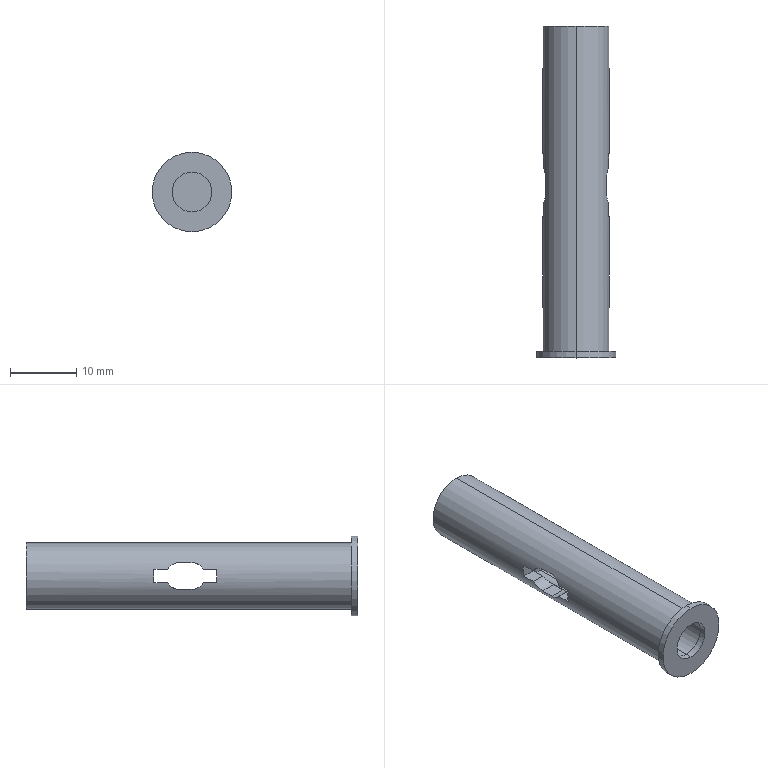Part | SolidWorks | features ICE 3, Revolution 1 | 1 solid | 37 faces | box 12 x 50 x 12 mm | volume 2925 mm3 | plane 21 | cylinder 16 | commonest cylinder face diameters 4 x8 6 x2 6.05 x2 10 x2 12 x2
STEP:
#1=CARTESIAN_POINT('',(0.,1.,-3.));
#2=VERTEX_POINT('',#1);
#3=CARTESIAN_POINT('',(0.,1.,3.));
#4=VERTEX_POINT('',#3);
#5=CARTESIAN_POINT('',(0.,1.,0.));
#6=DIRECTION('',(0.,1.,0.));
#7=DIRECTION('',(0.,0.,1.));
#8=AXIS2_PLACEMENT_3D('',#5,#6,#7);
#9=CIRCLE('',#8,3.);
#10=EDGE_CURVE('',#2,#4,#9,.T.);
#11=ORIENTED_EDGE('',*,*,#10,.T.);
#12=CARTESIAN_POINT('',(0.,0.,3.));
#13=VERTEX_POINT('',#12);
#14=CARTESIAN_POINT('',(0.,1.,3.));
#15=DIRECTION('',(0.,-1.,0.));
#16=VECTOR('',#15,1000.);
#17=LINE('',#14,#16);
#18=EDGE_CURVE('',#4,#13,#17,.T.);
#19=ORIENTED_EDGE('',*,*,#18,.T.);
#20=CARTESIAN_POINT('',(0.,0.,-3.));
#21=VERTEX_POINT('',#20);
#22=CARTESIAN_POINT('',(0.,0.,0.));
#23=DIRECTION('',(0.,1.,0.));
#24=DIRECTION('',(0.,0.,1.));
#25=AXIS2_PLACEMENT_3D('',#22,#23,#24);
#26=CIRCLE('',#25,3.);
#27=EDGE_CURVE('',#21,#13,#26,.T.);
#28=ORIENTED_EDGE('',*,*,#27,.F.);
#29=CARTESIAN_POINT('',(0.,1.,-3.));
#30=DIRECTION('',(0.,-1.,0.));
#31=VECTOR('',#30,1000.);
#32=LINE('',#29,#31);
#33=EDGE_CURVE('',#2,#21,#32,.T.);
#34=ORIENTED_EDGE('',*,*,#33,.F.);
#35=EDGE_LOOP('',(#11,#19,#28,#34));
#36=FACE_OUTER_BOUND('',#35,.T.);
#37=CARTESIAN_POINT('',(0.,1.,0.));
#38=DIRECTION('',(0.,-1.,0.));
#39=DIRECTION('',(0.,0.,-1.));
#40=AXIS2_PLACEMENT_3D('',#37,#38,#39);
#41=CYLINDRICAL_SURFACE('',#40,3.);
#42=ADVANCED_FACE('',(#36),#41,.F.);
#43=CARTESIAN_POINT('',(0.,1.,6.));
#44=VERTEX_POINT('',#43);
#45=CARTESIAN_POINT('',(0.,1.,-6.));
#46=VERTEX_POINT('',#45);
#47=CARTESIAN_POINT('',(0.,1.,0.));
#48=DIRECTION('',(0.,1.,0.));
#49=DIRECTION('',(0.,0.,1.));
#50=AXIS2_PLACEMENT_3D('',#47,#48,#49);
#51=CIRCLE('',#50,6.);
#52=EDGE_CURVE('',#44,#46,#51,.T.);
#53=ORIENTED_EDGE('',*,*,#52,.F.);
#54=CARTESIAN_POINT('',(0.,0.,6.));
#55=VERTEX_POINT('',#54);
#56=CARTESIAN_POINT('',(0.,1.,6.));
#57=DIRECTION('',(0.,-1.,0.));
#58=VECTOR('',#57,1000.);
#59=LINE('',#56,#58);
#60=EDGE_CURVE('',#44,#55,#59,.T.);
#61=ORIENTED_EDGE('',*,*,#60,.T.);
#62=CARTESIAN_POINT('',(0.,0.,-6.));
#63=VERTEX_POINT('',#62);
#64=CARTESIAN_POINT('',(0.,0.,0.));
#65=DIRECTION('',(0.,1.,0.));
#66=DIRECTION('',(0.,0.,1.));
#67=AXIS2_PLACEMENT_3D('',#64,#65,#66);
#68=CIRCLE('',#67,6.);
#69=EDGE_CURVE('',#55,#63,#68,.T.);
#70=ORIENTED_EDGE('',*,*,#69,.T.);
#71=CARTESIAN_POINT('',(0.,1.,-6.));
#72=DIRECTION('',(0.,-1.,0.));
#73=VECTOR('',#72,1000.);
#74=LINE('',#71,#73);
#75=EDGE_CURVE('',#46,#63,#74,.T.);
#76=ORIENTED_EDGE('',*,*,#75,.F.);
#77=EDGE_LOOP('',(#53,#61,#70,#76));
#78=FACE_OUTER_BOUND('',#77,.T.);
#79=CARTESIAN_POINT('',(0.,1.,0.));
#80=DIRECTION('',(0.,-1.,0.));
#81=DIRECTION('',(0.,0.,-1.));
#82=AXIS2_PLACEMENT_3D('',#79,#80,#81);
#83=CYLINDRICAL_SURFACE('',#82,6.);
#84=ADVANCED_FACE('',(#78),#83,.T.);
#85=CARTESIAN_POINT('',(4.899,30.732,-1.));
#86=VERTEX_POINT('',#85);
#87=CARTESIAN_POINT('',(4.899,30.732,1.));
#88=VERTEX_POINT('',#87);
#89=CARTESIAN_POINT('',(0.,30.732,0.));
#90=DIRECTION('',(0.,-1.,0.));
#91=DIRECTION('',(0.,0.,1.));
#92=AXIS2_PLACEMENT_3D('',#89,#90,#91);
#93=CIRCLE('',#92,5.);
#94=EDGE_CURVE('',#86,#88,#93,.T.);
#95=ORIENTED_EDGE('',*,*,#94,.F.);
#96=CARTESIAN_POINT('',(4.899,28.732,-1.));
#97=VERTEX_POINT('',#96);
#98=CARTESIAN_POINT('',(4.899,-0.7297,-1.));
#99=DIRECTION('',(0.,1.,0.));
#100=VECTOR('',#99,1000.);
#101=LINE('',#98,#100);
#102=EDGE_CURVE('',#97,#86,#101,.T.);
#103=ORIENTED_EDGE('',*,*,#102,.F.);
#104=CARTESIAN_POINT('',(4.583,27.,-2.));
#105=VERTEX_POINT('',#104);
#106=CARTESIAN_POINT('',(4.583,27.,-2.));
#107=CARTESIAN_POINT('',(4.583,27.179,-2.));
#108=CARTESIAN_POINT('',(4.593,27.353,-1.977));
#109=CARTESIAN_POINT('',(4.631,27.692,-1.885));
#110=CARTESIAN_POINT('',(4.659,27.855,-1.816));
#111=CARTESIAN_POINT('',(4.724,28.155,-1.642));
#112=CARTESIAN_POINT('',(4.761,28.295,-1.534));
#113=CARTESIAN_POINT('',(4.832,28.538,-1.29));
#114=CARTESIAN_POINT('',(4.868,28.645,-1.15));
#115=CARTESIAN_POINT('',(4.899,28.732,-1.));
#116=B_SPLINE_CURVE_WITH_KNOTS('',3,(#106,#107,#108,#109,#110,#111,#112,#113,#114,#115),.UNSPECIFIED.,.F.,.F.,(4,2,2,2,4),(0.,0.0005276,0.001055,0.001583,0.00211),.UNSPECIFIED.);
#117=EDGE_CURVE('',#105,#97,#116,.T.);
#118=ORIENTED_EDGE('',*,*,#117,.F.);
#119=CARTESIAN_POINT('',(4.583,25.,-2.));
#120=VERTEX_POINT('',#119);
#121=CARTESIAN_POINT('',(4.583,-0.7297,-2.));
#122=DIRECTION('',(0.,1.,0.));
#123=VECTOR('',#122,1000.);
#124=LINE('',#121,#123);
#125=EDGE_CURVE('',#120,#105,#124,.T.);
#126=ORIENTED_EDGE('',*,*,#125,.F.);
#127=CARTESIAN_POINT('',(4.899,23.268,-1.));
#128=VERTEX_POINT('',#127);
#129=CARTESIAN_POINT('',(4.899,23.268,-1.));
#130=CARTESIAN_POINT('',(4.868,23.355,-1.15));
#131=CARTESIAN_POINT('',(4.832,23.462,-1.29));
#132=CARTESIAN_POINT('',(4.76,23.706,-1.535));
#133=CARTESIAN_POINT('',(4.724,23.842,-1.64));
#134=CARTESIAN_POINT('',(4.659,24.145,-1.817));
#135=CARTESIAN_POINT('',(4.632,24.305,-1.884));
#136=CARTESIAN_POINT('',(4.593,24.643,-1.976));
#137=CARTESIAN_POINT('',(4.583,24.821,-2.));
#138=CARTESIAN_POINT('',(4.583,25.,-2.));
#139=B_SPLINE_CURVE_WITH_KNOTS('',3,(#129,#130,#131,#132,#133,#134,#135,#136,#137,#138),.UNSPECIFIED.,.F.,.F.,(4,2,2,2,4),(0.004207,0.004735,0.005262,0.005789,0.006317),.UNSPECIFIED.);
#140=EDGE_CURVE('',#128,#120,#139,.T.);
#141=ORIENTED_EDGE('',*,*,#140,.F.);
#142=CARTESIAN_POINT('',(4.899,21.268,-1.));
#143=VERTEX_POINT('',#142);
#144=CARTESIAN_POINT('',(4.899,-0.7297,-1.));
#145=DIRECTION('',(0.,1.,0.));
#146=VECTOR('',#145,1000.);
#147=LINE('',#144,#146);
#148=EDGE_CURVE('',#143,#128,#147,.T.);
#149=ORIENTED_EDGE('',*,*,#148,.F.);
#150=CARTESIAN_POINT('',(4.899,21.268,1.));
#151=VERTEX_POINT('',#150);
#152=CARTESIAN_POINT('',(0.,21.268,0.));
#153=DIRECTION('',(0.,1.,0.));
#154=DIRECTION('',(0.,0.,-1.));
#155=AXIS2_PLACEMENT_3D('',#152,#153,#154);
#156=CIRCLE('',#155,5.);
#157=EDGE_CURVE('',#151,#143,#156,.T.);
#158=ORIENTED_EDGE('',*,*,#157,.F.);
#159=CARTESIAN_POINT('',(4.899,23.268,1.));
#160=VERTEX_POINT('',#159);
#161=CARTESIAN_POINT('',(4.899,-0.7297,1.));
#162=DIRECTION('',(0.,-1.,0.));
#163=VECTOR('',#162,1000.);
#164=LINE('',#161,#163);
#165=EDGE_CURVE('',#160,#151,#164,.T.);
#166=ORIENTED_EDGE('',*,*,#165,.F.);
#167=CARTESIAN_POINT('',(4.583,25.,2.));
#168=VERTEX_POINT('',#167);
#169=CARTESIAN_POINT('',(4.583,25.,2.));
#170=CARTESIAN_POINT('',(4.583,24.821,2.));
#171=CARTESIAN_POINT('',(4.593,24.647,1.977));
#172=CARTESIAN_POINT('',(4.631,24.308,1.885));
#173=CARTESIAN_POINT('',(4.659,24.145,1.816));
#174=CARTESIAN_POINT('',(4.724,23.845,1.642));
#175=CARTESIAN_POINT('',(4.761,23.705,1.534));
#176=CARTESIAN_POINT('',(4.832,23.462,1.29));
#177=CARTESIAN_POINT('',(4.868,23.355,1.15));
#178=CARTESIAN_POINT('',(4.899,23.268,1.));
#179=B_SPLINE_CURVE_WITH_KNOTS('',3,(#169,#170,#171,#172,#173,#174,#175,#176,#177,#178),.UNSPECIFIED.,.F.,.F.,(4,2,2,2,4),(0.,0.0005276,0.001055,0.001583,0.00211),.UNSPECIFIED.);
#180=EDGE_CURVE('',#168,#160,#179,.T.);
#181=ORIENTED_EDGE('',*,*,#180,.F.);
#182=CARTESIAN_POINT('',(4.583,27.,2.));
#183=VERTEX_POINT('',#182);
#184=CARTESIAN_POINT('',(4.583,-0.7297,2.));
#185=DIRECTION('',(0.,-1.,0.));
#186=VECTOR('',#185,1000.);
#187=LINE('',#184,#186);
#188=EDGE_CURVE('',#183,#168,#187,.T.);
#189=ORIENTED_EDGE('',*,*,#188,.F.);
#190=CARTESIAN_POINT('',(4.899,28.732,1.));
#191=VERTEX_POINT('',#190);
#192=CARTESIAN_POINT('',(4.899,28.732,1.));
#193=CARTESIAN_POINT('',(4.868,28.645,1.15));
#194=CARTESIAN_POINT('',(4.832,28.538,1.29));
#195=CARTESIAN_POINT('',(4.76,28.294,1.535));
#196=CARTESIAN_POINT('',(4.724,28.158,1.64));
#197=CARTESIAN_POINT('',(4.659,27.855,1.817));
#198=CARTESIAN_POINT('',(4.632,27.695,1.884));
#199=CARTESIAN_POINT('',(4.593,27.357,1.976));
#200=CARTESIAN_POINT('',(4.583,27.179,2.));
#201=CARTESIAN_POINT('',(4.583,27.,2.));
#202=B_SPLINE_CURVE_WITH_KNOTS('',3,(#192,#193,#194,#195,#196,#197,#198,#199,#200,#201),.UNSPECIFIED.,.F.,.F.,(4,2,2,2,4),(0.004207,0.004735,0.005262,0.005789,0.006317),.UNSPECIFIED.);
#203=EDGE_CURVE('',#191,#183,#202,.T.);
#204=ORIENTED_EDGE('',*,*,#203,.F.);
#205=CARTESIAN_POINT('',(4.899,-0.7297,1.));
#206=DIRECTION('',(0.,-1.,0.));
#207=VECTOR('',#206,1000.);
#208=LINE('',#205,#207);
#209=EDGE_CURVE('',#88,#191,#208,.T.);
#210=ORIENTED_EDGE('',*,*,#209,.F.);
#211=EDGE_LOOP('',(#95,#103,#118,#126,#141,#149,#158,#166,#181,#189,#204,#210));
#212=FACE_BOUND('',#211,.T.);
#213=CARTESIAN_POINT('',(0.,50.,-5.));
#214=VERTEX_POINT('',#213);
#215=CARTESIAN_POINT('',(0.,50.,5.));
#216=VERTEX_POINT('',#215);
#217=CARTESIAN_POINT('',(0.,50.,0.));
#218=DIRECTION('',(0.,-1.,0.));
#219=DIRECTION('',(0.,0.,-1.));
#220=AXIS2_PLACEMENT_3D('',#217,#218,#219);
#221=CIRCLE('',#220,5.);
#222=EDGE_CURVE('',#214,#216,#221,.T.);
#223=ORIENTED_EDGE('',*,*,#222,.T.);
#224=CARTESIAN_POINT('',(0.,1.,5.));
#225=VERTEX_POINT('',#224);
#226=CARTESIAN_POINT('',(0.,-0.7297,5.));
#227=DIRECTION('',(0.,-1.,0.));
#228=VECTOR('',#227,1000.);
#229=LINE('',#226,#228);
#230=EDGE_CURVE('',#216,#225,#229,.T.);
#231=ORIENTED_EDGE('',*,*,#230,.T.);
#232=CARTESIAN_POINT('',(0.,1.,-5.));
#233=VERTEX_POINT('',#232);
#234=CARTESIAN_POINT('',(0.,1.,0.));
#235=DIRECTION('',(0.,-1.,0.));
#236=DIRECTION('',(0.,0.,1.));
#237=AXIS2_PLACEMENT_3D('',#234,#235,#236);
#238=CIRCLE('',#237,5.);
#239=EDGE_CURVE('',#233,#225,#238,.T.);
#240=ORIENTED_EDGE('',*,*,#239,.F.);
#241=CARTESIAN_POINT('',(0.,-0.7297,-5.));
#242=DIRECTION('',(0.,-1.,0.));
#243=VECTOR('',#242,1000.);
#244=LINE('',#241,#243);
#245=EDGE_CURVE('',#214,#233,#244,.T.);
#246=ORIENTED_EDGE('',*,*,#245,.F.);
#247=EDGE_LOOP('',(#223,#231,#240,#246));
#248=FACE_OUTER_BOUND('',#247,.T.);
#249=CARTESIAN_POINT('',(0.,-0.7297,0.));
#250=DIRECTION('',(0.,-1.,0.));
#251=DIRECTION('',(0.,0.,-1.));
#252=AXIS2_PLACEMENT_3D('',#249,#250,#251);
#253=CYLINDRICAL_SURFACE('',#252,5.);
#254=ADVANCED_FACE('',(#212,#248),#253,.T.);
#255=CARTESIAN_POINT('',(-2.855,30.732,1.));
#256=VERTEX_POINT('',#255);
#257=CARTESIAN_POINT('',(-2.855,28.732,1.));
#258=VERTEX_POINT('',#257);
#259=CARTESIAN_POINT('',(-2.855,-0.7297,1.));
#260=DIRECTION('',(0.,-1.,0.));
#261=VECTOR('',#260,1000.);
#262=LINE('',#259,#261);
#263=EDGE_CURVE('',#256,#258,#262,.T.);
#264=ORIENTED_EDGE('',*,*,#263,.F.);
#265=CARTESIAN_POINT('',(-2.855,30.732,-1.));
#266=VERTEX_POINT('',#265);
#267=CARTESIAN_POINT('',(0.,30.732,0.));
#268=DIRECTION('',(0.,1.,0.));
#269=DIRECTION('',(0.,0.,1.));
#270=AXIS2_PLACEMENT_3D('',#267,#268,#269);
#271=CIRCLE('',#270,3.025);
#272=EDGE_CURVE('',#266,#256,#271,.T.);
#273=ORIENTED_EDGE('',*,*,#272,.F.);
#274=CARTESIAN_POINT('',(-2.855,28.732,-1.));
#275=VERTEX_POINT('',#274);
#276=CARTESIAN_POINT('',(-2.855,-0.7297,-1.));
#277=DIRECTION('',(0.,1.,0.));
#278=VECTOR('',#277,1000.);
#279=LINE('',#276,#278);
#280=EDGE_CURVE('',#275,#266,#279,.T.);
#281=ORIENTED_EDGE('',*,*,#280,.F.);
#282=CARTESIAN_POINT('',(-2.269,27.,-2.));
#283=VERTEX_POINT('',#282);
#284=CARTESIAN_POINT('',(-2.269,27.,-2.));
#285=CARTESIAN_POINT('',(-2.269,27.184,-2.));
#286=CARTESIAN_POINT('',(-2.292,27.362,-1.975));
#287=CARTESIAN_POINT('',(-2.371,27.707,-1.879));
#288=CARTESIAN_POINT('',(-2.426,27.867,-1.81));
#289=CARTESIAN_POINT('',(-2.547,28.164,-1.635));
#290=CARTESIAN_POINT('',(-2.613,28.299,-1.53));
#291=CARTESIAN_POINT('',(-2.74,28.539,-1.288));
#292=CARTESIAN_POINT('',(-2.803,28.646,-1.15));
#293=CARTESIAN_POINT('',(-2.855,28.732,-1.));
#294=B_SPLINE_CURVE_WITH_KNOTS('',3,(#284,#285,#286,#287,#288,#289,#290,#291,#292,#293),.UNSPECIFIED.,.F.,.F.,(4,2,2,2,4),(0.,0.0005429,0.001086,0.001629,0.002172),.UNSPECIFIED.);
#295=EDGE_CURVE('',#283,#275,#294,.T.);
#296=ORIENTED_EDGE('',*,*,#295,.F.);
#297=CARTESIAN_POINT('',(-2.269,25.,-2.));
#298=VERTEX_POINT('',#297);
#299=CARTESIAN_POINT('',(-2.269,-0.7297,-2.));
#300=DIRECTION('',(0.,1.,0.));
#301=VECTOR('',#300,1000.);
#302=LINE('',#299,#301);
#303=EDGE_CURVE('',#298,#283,#302,.T.);
#304=ORIENTED_EDGE('',*,*,#303,.F.);
#305=CARTESIAN_POINT('',(-2.855,23.268,-1.));
#306=VERTEX_POINT('',#305);
#307=CARTESIAN_POINT('',(-2.855,23.268,-1.));
#308=CARTESIAN_POINT('',(-2.749,23.442,-1.302));
#309=CARTESIAN_POINT('',(-2.607,23.69,-1.549));
#310=CARTESIAN_POINT('',(-2.427,24.131,-1.809));
#311=CARTESIAN_POINT('',(-2.371,24.292,-1.879));
#312=CARTESIAN_POINT('',(-2.293,24.635,-1.975));
#313=CARTESIAN_POINT('',(-2.269,24.816,-2.));
#314=CARTESIAN_POINT('',(-2.269,25.,-2.));
#315=B_SPLINE_CURVE_WITH_KNOTS('',3,(#307,#308,#309,#310,#311,#312,#313,#314),.UNSPECIFIED.,.F.,.F.,(4,2,2,4),(0.004288,0.005372,0.005913,0.006455),.UNSPECIFIED.);
#316=EDGE_CURVE('',#306,#298,#315,.T.);
#317=ORIENTED_EDGE('',*,*,#316,.F.);
#318=CARTESIAN_POINT('',(-2.855,21.268,-1.));
#319=VERTEX_POINT('',#318);
#320=CARTESIAN_POINT('',(-2.855,-0.7297,-1.));
#321=DIRECTION('',(0.,1.,0.));
#322=VECTOR('',#321,1000.);
#323=LINE('',#320,#322);
#324=EDGE_CURVE('',#319,#306,#323,.T.);
#325=ORIENTED_EDGE('',*,*,#324,.F.);
#326=CARTESIAN_POINT('',(-2.855,21.268,1.));
#327=VERTEX_POINT('',#326);
#328=CARTESIAN_POINT('',(0.,21.268,0.));
#329=DIRECTION('',(0.,-1.,0.));
#330=DIRECTION('',(0.,0.,-1.));
#331=AXIS2_PLACEMENT_3D('',#328,#329,#330);
#332=CIRCLE('',#331,3.025);
#333=EDGE_CURVE('',#327,#319,#332,.T.);
#334=ORIENTED_EDGE('',*,*,#333,.F.);
#335=CARTESIAN_POINT('',(-2.855,23.268,1.));
#336=VERTEX_POINT('',#335);
#337=CARTESIAN_POINT('',(-2.855,-0.7297,1.));
#338=DIRECTION('',(0.,-1.,0.));
#339=VECTOR('',#338,1000.);
#340=LINE('',#337,#339);
#341=EDGE_CURVE('',#336,#327,#340,.T.);
#342=ORIENTED_EDGE('',*,*,#341,.F.);
#343=CARTESIAN_POINT('',(-2.269,25.,2.));
#344=VERTEX_POINT('',#343);
#345=CARTESIAN_POINT('',(-2.269,25.,2.));
#346=CARTESIAN_POINT('',(-2.269,24.816,2.));
#347=CARTESIAN_POINT('',(-2.292,24.638,1.975));
#348=CARTESIAN_POINT('',(-2.371,24.293,1.879));
#349=CARTESIAN_POINT('',(-2.426,24.133,1.81));
#350=CARTESIAN_POINT('',(-2.547,23.836,1.635));
#351=CARTESIAN_POINT('',(-2.613,23.701,1.53));
#352=CARTESIAN_POINT('',(-2.74,23.461,1.288));
#353=CARTESIAN_POINT('',(-2.803,23.354,1.15));
#354=CARTESIAN_POINT('',(-2.855,23.268,1.));
#355=B_SPLINE_CURVE_WITH_KNOTS('',3,(#345,#346,#347,#348,#349,#350,#351,#352,#353,#354),.UNSPECIFIED.,.F.,.F.,(4,2,2,2,4),(0.,0.0005429,0.001086,0.001629,0.002172),.UNSPECIFIED.);
#356=EDGE_CURVE('',#344,#336,#355,.T.);
#357=ORIENTED_EDGE('',*,*,#356,.F.);
#358=CARTESIAN_POINT('',(-2.269,27.,2.));
#359=VERTEX_POINT('',#358);
#360=CARTESIAN_POINT('',(-2.269,-0.7297,2.));
#361=DIRECTION('',(0.,-1.,0.));
#362=VECTOR('',#361,1000.);
#363=LINE('',#360,#362);
#364=EDGE_CURVE('',#359,#344,#363,.T.);
#365=ORIENTED_EDGE('',*,*,#364,.F.);
#366=CARTESIAN_POINT('',(-2.855,28.732,1.));
#367=CARTESIAN_POINT('',(-2.749,28.558,1.302));
#368=CARTESIAN_POINT('',(-2.607,28.31,1.549));
#369=CARTESIAN_POINT('',(-2.427,27.869,1.809));
#370=CARTESIAN_POINT('',(-2.371,27.708,1.879));
#371=CARTESIAN_POINT('',(-2.293,27.365,1.975));
#372=CARTESIAN_POINT('',(-2.269,27.184,2.));
#373=CARTESIAN_POINT('',(-2.269,27.,2.));
#374=B_SPLINE_CURVE_WITH_KNOTS('',3,(#366,#367,#368,#369,#370,#371,#372,#373),.UNSPECIFIED.,.F.,.F.,(4,2,2,4),(0.004288,0.005372,0.005913,0.006455),.UNSPECIFIED.);
#375=EDGE_CURVE('',#258,#359,#374,.T.);
#376=ORIENTED_EDGE('',*,*,#375,.F.);
#377=EDGE_LOOP('',(#264,#273,#281,#296,#304,#317,#325,#334,#342,#357,#365,#376));
#378=FACE_BOUND('',#377,.T.);
#379=CARTESIAN_POINT('',(0.,32.1,3.025));
#380=VERTEX_POINT('',#379);
#381=CARTESIAN_POINT('',(0.,32.1,-3.025));
#382=VERTEX_POINT('',#381);
#383=CARTESIAN_POINT('',(0.,32.1,0.));
#384=DIRECTION('',(0.,-1.,0.));
#385=DIRECTION('',(0.,0.,-1.));
#386=AXIS2_PLACEMENT_3D('',#383,#384,#385);
#387=CIRCLE('',#386,3.025);
#388=EDGE_CURVE('',#380,#382,#387,.T.);
#389=ORIENTED_EDGE('',*,*,#388,.F.);
#390=CARTESIAN_POINT('',(0.,1.,3.025));
#391=VERTEX_POINT('',#390);
#392=CARTESIAN_POINT('',(0.,-0.7297,3.025));
#393=DIRECTION('',(0.,-1.,0.));
#394=VECTOR('',#393,1000.);
#395=LINE('',#392,#394);
#396=EDGE_CURVE('',#380,#391,#395,.T.);
#397=ORIENTED_EDGE('',*,*,#396,.T.);
#398=CARTESIAN_POINT('',(0.,1.,-3.025));
#399=VERTEX_POINT('',#398);
#400=CARTESIAN_POINT('',(0.,1.,0.));
#401=DIRECTION('',(0.,1.,0.));
#402=DIRECTION('',(0.,0.,1.));
#403=AXIS2_PLACEMENT_3D('',#400,#401,#402);
#404=CIRCLE('',#403,3.025);
#405=EDGE_CURVE('',#399,#391,#404,.T.);
#406=ORIENTED_EDGE('',*,*,#405,.F.);
#407=CARTESIAN_POINT('',(0.,-0.7297,-3.025));
#408=DIRECTION('',(0.,-1.,0.));
#409=VECTOR('',#408,1000.);
#410=LINE('',#407,#409);
#411=EDGE_CURVE('',#382,#399,#410,.T.);
#412=ORIENTED_EDGE('',*,*,#411,.F.);
#413=EDGE_LOOP('',(#389,#397,#406,#412));
#414=FACE_OUTER_BOUND('',#413,.T.);
#415=CARTESIAN_POINT('',(0.,-0.7297,0.));
#416=DIRECTION('',(0.,-1.,0.));
#417=DIRECTION('',(0.,0.,-1.));
#418=AXIS2_PLACEMENT_3D('',#415,#416,#417);
#419=CYLINDRICAL_SURFACE('',#418,3.025);
#420=ADVANCED_FACE('',(#378,#414),#419,.F.);
#421=ORIENTED_EDGE('',*,*,#180,.T.);
#422=CARTESIAN_POINT('',(2.855,23.268,1.));
#423=VERTEX_POINT('',#422);
#424=CARTESIAN_POINT('',(-5.,23.268,1.));
#425=DIRECTION('',(-1.,0.,0.));
#426=VECTOR('',#425,1000.);
#427=LINE('',#424,#426);
#428=EDGE_CURVE('',#160,#423,#427,.T.);
#429=ORIENTED_EDGE('',*,*,#428,.T.);
#430=CARTESIAN_POINT('',(2.269,25.,2.));
#431=VERTEX_POINT('',#430);
#432=CARTESIAN_POINT('',(2.855,23.268,1.));
#433=CARTESIAN_POINT('',(2.749,23.442,1.302));
#434=CARTESIAN_POINT('',(2.607,23.69,1.549));
#435=CARTESIAN_POINT('',(2.427,24.131,1.809));
#436=CARTESIAN_POINT('',(2.371,24.292,1.879));
#437=CARTESIAN_POINT('',(2.293,24.635,1.975));
#438=CARTESIAN_POINT('',(2.269,24.816,2.));
#439=CARTESIAN_POINT('',(2.269,25.,2.));
#440=B_SPLINE_CURVE_WITH_KNOTS('',3,(#432,#433,#434,#435,#436,#437,#438,#439),.UNSPECIFIED.,.F.,.F.,(4,2,2,4),(0.004288,0.005372,0.005913,0.006455),.UNSPECIFIED.);
#441=EDGE_CURVE('',#423,#431,#440,.T.);
#442=ORIENTED_EDGE('',*,*,#441,.T.);
#443=CARTESIAN_POINT('',(-5.,25.,2.));
#444=DIRECTION('',(1.,0.,0.));
#445=VECTOR('',#444,1000.);
#446=LINE('',#443,#445);
#447=EDGE_CURVE('',#431,#168,#446,.T.);
#448=ORIENTED_EDGE('',*,*,#447,.T.);
#449=EDGE_LOOP('',(#421,#429,#442,#448));
#450=FACE_OUTER_BOUND('',#449,.T.);
#451=CARTESIAN_POINT('',(-5.,25.,0.));
#452=DIRECTION('',(1.,0.,0.));
#453=DIRECTION('',(0.,0.,-1.));
#454=AXIS2_PLACEMENT_3D('',#451,#452,#453);
#455=CYLINDRICAL_SURFACE('',#454,2.);
#456=ADVANCED_FACE('',(#450),#455,.F.);
#457=CARTESIAN_POINT('',(2.269,27.,2.));
#458=VERTEX_POINT('',#457);
#459=CARTESIAN_POINT('',(2.855,28.732,1.));
#460=VERTEX_POINT('',#459);
#461=CARTESIAN_POINT('',(2.269,27.,2.));
#462=CARTESIAN_POINT('',(2.269,27.184,2.));
#463=CARTESIAN_POINT('',(2.292,27.362,1.975));
#464=CARTESIAN_POINT('',(2.371,27.707,1.879));
#465=CARTESIAN_POINT('',(2.426,27.867,1.81));
#466=CARTESIAN_POINT('',(2.547,28.164,1.635));
#467=CARTESIAN_POINT('',(2.613,28.299,1.53));
#468=CARTESIAN_POINT('',(2.74,28.539,1.288));
#469=CARTESIAN_POINT('',(2.803,28.646,1.15));
#470=CARTESIAN_POINT('',(2.855,28.732,1.));
#471=B_SPLINE_CURVE_WITH_KNOTS('',3,(#461,#462,#463,#464,#465,#466,#467,#468,#469,#470),.UNSPECIFIED.,.F.,.F.,(4,2,2,2,4),(0.,0.0005429,0.001086,0.001629,0.002172),.UNSPECIFIED.);
#472=EDGE_CURVE('',#458,#460,#471,.T.);
#473=ORIENTED_EDGE('',*,*,#472,.T.);
#474=CARTESIAN_POINT('',(-5.,28.732,1.));
#475=DIRECTION('',(1.,0.,0.));
#476=VECTOR('',#475,1000.);
#477=LINE('',#474,#476);
#478=EDGE_CURVE('',#460,#191,#477,.T.);
#479=ORIENTED_EDGE('',*,*,#478,.T.);
#480=ORIENTED_EDGE('',*,*,#203,.T.);
#481=CARTESIAN_POINT('',(-5.,27.,2.));
#482=DIRECTION('',(1.,0.,0.));
#483=VECTOR('',#482,1000.);
#484=LINE('',#481,#483);
#485=EDGE_CURVE('',#458,#183,#484,.T.);
#486=ORIENTED_EDGE('',*,*,#485,.F.);
#487=EDGE_LOOP('',(#473,#479,#480,#486));
#488=FACE_OUTER_BOUND('',#487,.T.);
#489=CARTESIAN_POINT('',(-5.,27.,0.));
#490=DIRECTION('',(1.,0.,0.));
#491=DIRECTION('',(0.,0.,-1.));
#492=AXIS2_PLACEMENT_3D('',#489,#490,#491);
#493=CYLINDRICAL_SURFACE('',#492,2.);
#494=ADVANCED_FACE('',(#488),#493,.F.);
#495=CARTESIAN_POINT('',(-4.583,27.,2.));
#496=VERTEX_POINT('',#495);
#497=CARTESIAN_POINT('',(-4.899,28.732,1.));
#498=VERTEX_POINT('',#497);
#499=CARTESIAN_POINT('',(-4.583,27.,2.));
#500=CARTESIAN_POINT('',(-4.583,27.179,2.));
#501=CARTESIAN_POINT('',(-4.593,27.353,1.977));
#502=CARTESIAN_POINT('',(-4.631,27.692,1.885));
#503=CARTESIAN_POINT('',(-4.659,27.855,1.816));
#504=CARTESIAN_POINT('',(-4.724,28.155,1.642));
#505=CARTESIAN_POINT('',(-4.761,28.295,1.534));
#506=CARTESIAN_POINT('',(-4.832,28.538,1.29));
#507=CARTESIAN_POINT('',(-4.868,28.645,1.15));
#508=CARTESIAN_POINT('',(-4.899,28.732,1.));
#509=B_SPLINE_CURVE_WITH_KNOTS('',3,(#499,#500,#501,#502,#503,#504,#505,#506,#507,#508),.UNSPECIFIED.,.F.,.F.,(4,2,2,2,4),(0.,0.0005276,0.001055,0.001583,0.00211),.UNSPECIFIED.);
#510=EDGE_CURVE('',#496,#498,#509,.T.);
#511=ORIENTED_EDGE('',*,*,#510,.T.);
#512=CARTESIAN_POINT('',(-5.,28.732,1.));
#513=DIRECTION('',(1.,0.,0.));
#514=VECTOR('',#513,1000.);
#515=LINE('',#512,#514);
#516=EDGE_CURVE('',#498,#258,#515,.T.);
#517=ORIENTED_EDGE('',*,*,#516,.T.);
#518=ORIENTED_EDGE('',*,*,#375,.T.);
#519=CARTESIAN_POINT('',(-5.,27.,2.));
#520=DIRECTION('',(1.,0.,0.));
#521=VECTOR('',#520,1000.);
#522=LINE('',#519,#521);
#523=EDGE_CURVE('',#496,#359,#522,.T.);
#524=ORIENTED_EDGE('',*,*,#523,.F.);
#525=EDGE_LOOP('',(#511,#517,#518,#524));
#526=FACE_OUTER_BOUND('',#525,.T.);
#527=CARTESIAN_POINT('',(-5.,27.,0.));
#528=DIRECTION('',(1.,0.,0.));
#529=DIRECTION('',(0.,0.,-1.));
#530=AXIS2_PLACEMENT_3D('',#527,#528,#529);
#531=CYLINDRICAL_SURFACE('',#530,2.);
#532=ADVANCED_FACE('',(#526),#531,.F.);
#533=ORIENTED_EDGE('',*,*,#356,.T.);
#534=CARTESIAN_POINT('',(-4.899,23.268,1.));
#535=VERTEX_POINT('',#534);
#536=CARTESIAN_POINT('',(-5.,23.268,1.));
#537=DIRECTION('',(-1.,0.,0.));
#538=VECTOR('',#537,1000.);
#539=LINE('',#536,#538);
#540=EDGE_CURVE('',#336,#535,#539,.T.);
#541=ORIENTED_EDGE('',*,*,#540,.T.);
#542=CARTESIAN_POINT('',(-4.583,25.,2.));
#543=VERTEX_POINT('',#542);
#544=CARTESIAN_POINT('',(-4.899,23.268,1.));
#545=CARTESIAN_POINT('',(-4.868,23.355,1.15));
#546=CARTESIAN_POINT('',(-4.832,23.462,1.29));
#547=CARTESIAN_POINT('',(-4.76,23.706,1.535));
#548=CARTESIAN_POINT('',(-4.724,23.842,1.64));
#549=CARTESIAN_POINT('',(-4.659,24.145,1.817));
#550=CARTESIAN_POINT('',(-4.632,24.305,1.884));
#551=CARTESIAN_POINT('',(-4.593,24.643,1.976));
#552=CARTESIAN_POINT('',(-4.583,24.821,2.));
#553=CARTESIAN_POINT('',(-4.583,25.,2.));
#554=B_SPLINE_CURVE_WITH_KNOTS('',3,(#544,#545,#546,#547,#548,#549,#550,#551,#552,#553),.UNSPECIFIED.,.F.,.F.,(4,2,2,2,4),(0.004207,0.004735,0.005262,0.005789,0.006317),.UNSPECIFIED.);
#555=EDGE_CURVE('',#535,#543,#554,.T.);
#556=ORIENTED_EDGE('',*,*,#555,.T.);
#557=CARTESIAN_POINT('',(-5.,25.,2.));
#558=DIRECTION('',(1.,0.,0.));
#559=VECTOR('',#558,1000.);
#560=LINE('',#557,#559);
#561=EDGE_CURVE('',#543,#344,#560,.T.);
#562=ORIENTED_EDGE('',*,*,#561,.T.);
#563=EDGE_LOOP('',(#533,#541,#556,#562));
#564=FACE_OUTER_BOUND('',#563,.T.);
#565=CARTESIAN_POINT('',(-5.,25.,0.));
#566=DIRECTION('',(1.,0.,0.));
#567=DIRECTION('',(0.,0.,-1.));
#568=AXIS2_PLACEMENT_3D('',#565,#566,#567);
#569=CYLINDRICAL_SURFACE('',#568,2.);
#570=ADVANCED_FACE('',(#564),#569,.F.);
#571=ORIENTED_EDGE('',*,*,#396,.F.);
#572=CARTESIAN_POINT('',(0.,32.1,0.));
#573=DIRECTION('',(0.,-1.,0.));
#574=DIRECTION('',(0.,0.,-1.));
#575=AXIS2_PLACEMENT_3D('',#572,#573,#574);
#576=CIRCLE('',#575,3.025);
#577=EDGE_CURVE('',#382,#380,#576,.T.);
#578=ORIENTED_EDGE('',*,*,#577,.F.);
#579=ORIENTED_EDGE('',*,*,#411,.T.);
#580=CARTESIAN_POINT('',(0.,1.,0.));
#581=DIRECTION('',(0.,1.,0.));
#582=DIRECTION('',(0.,0.,1.));
#583=AXIS2_PLACEMENT_3D('',#580,#581,#582);
#584=CIRCLE('',#583,3.025);
#585=EDGE_CURVE('',#391,#399,#584,.T.);
#586=ORIENTED_EDGE('',*,*,#585,.F.);
#587=EDGE_LOOP('',(#571,#578,#579,#586));
#588=FACE_OUTER_BOUND('',#587,.T.);
#589=CARTESIAN_POINT('',(2.855,30.732,1.));
#590=VERTEX_POINT('',#589);
#591=CARTESIAN_POINT('',(2.855,-0.7297,1.));
#592=DIRECTION('',(0.,1.,0.));
#593=VECTOR('',#592,1000.);
#594=LINE('',#591,#593);
#595=EDGE_CURVE('',#460,#590,#594,.T.);
#596=ORIENTED_EDGE('',*,*,#595,.F.);
#597=ORIENTED_EDGE('',*,*,#472,.F.);
#598=CARTESIAN_POINT('',(2.269,-0.7297,2.));
#599=DIRECTION('',(0.,1.,0.));
#600=VECTOR('',#599,1000.);
#601=LINE('',#598,#600);
#602=EDGE_CURVE('',#431,#458,#601,.T.);
#603=ORIENTED_EDGE('',*,*,#602,.F.);
#604=ORIENTED_EDGE('',*,*,#441,.F.);
#605=CARTESIAN_POINT('',(2.855,21.268,1.));
#606=VERTEX_POINT('',#605);
#607=CARTESIAN_POINT('',(2.855,-0.7297,1.));
#608=DIRECTION('',(0.,1.,0.));
#609=VECTOR('',#608,1000.);
#610=LINE('',#607,#609);
#611=EDGE_CURVE('',#606,#423,#610,.T.);
#612=ORIENTED_EDGE('',*,*,#611,.F.);
#613=CARTESIAN_POINT('',(2.855,21.268,-1.));
#614=VERTEX_POINT('',#613);
#615=CARTESIAN_POINT('',(0.,21.268,0.));
#616=DIRECTION('',(0.,-1.,0.));
#617=DIRECTION('',(0.,0.,-1.));
#618=AXIS2_PLACEMENT_3D('',#615,#616,#617);
#619=CIRCLE('',#618,3.025);
#620=EDGE_CURVE('',#614,#606,#619,.T.);
#621=ORIENTED_EDGE('',*,*,#620,.F.);
#622=CARTESIAN_POINT('',(2.855,23.268,-1.));
#623=VERTEX_POINT('',#622);
#624=CARTESIAN_POINT('',(2.855,-0.7297,-1.));
#625=DIRECTION('',(0.,-1.,0.));
#626=VECTOR('',#625,1000.);
#627=LINE('',#624,#626);
#628=EDGE_CURVE('',#623,#614,#627,.T.);
#629=ORIENTED_EDGE('',*,*,#628,.F.);
#630=CARTESIAN_POINT('',(2.269,25.,-2.));
#631=VERTEX_POINT('',#630);
#632=CARTESIAN_POINT('',(2.269,25.,-2.));
#633=CARTESIAN_POINT('',(2.269,24.816,-2.));
#634=CARTESIAN_POINT('',(2.292,24.638,-1.975));
#635=CARTESIAN_POINT('',(2.371,24.293,-1.879));
#636=CARTESIAN_POINT('',(2.426,24.133,-1.81));
#637=CARTESIAN_POINT('',(2.547,23.836,-1.635));
#638=CARTESIAN_POINT('',(2.613,23.701,-1.53));
#639=CARTESIAN_POINT('',(2.74,23.461,-1.288));
#640=CARTESIAN_POINT('',(2.803,23.354,-1.15));
#641=CARTESIAN_POINT('',(2.855,23.268,-1.));
#642=B_SPLINE_CURVE_WITH_KNOTS('',3,(#632,#633,#634,#635,#636,#637,#638,#639,#640,#641),.UNSPECIFIED.,.F.,.F.,(4,2,2,2,4),(0.,0.0005429,0.001086,0.001629,0.002172),.UNSPECIFIED.);
#643=EDGE_CURVE('',#631,#623,#642,.T.);
#644=ORIENTED_EDGE('',*,*,#643,.F.);
#645=CARTESIAN_POINT('',(2.269,27.,-2.));
#646=VERTEX_POINT('',#645);
#647=CARTESIAN_POINT('',(2.269,-0.7297,-2.));
#648=DIRECTION('',(0.,-1.,0.));
#649=VECTOR('',#648,1000.);
#650=LINE('',#647,#649);
#651=EDGE_CURVE('',#646,#631,#650,.T.);
#652=ORIENTED_EDGE('',*,*,#651,.F.);
#653=CARTESIAN_POINT('',(2.855,28.732,-1.));
#654=VERTEX_POINT('',#653);
#655=CARTESIAN_POINT('',(2.855,28.732,-1.));
#656=CARTESIAN_POINT('',(2.749,28.558,-1.302));
#657=CARTESIAN_POINT('',(2.607,28.31,-1.549));
#658=CARTESIAN_POINT('',(2.427,27.869,-1.809));
#659=CARTESIAN_POINT('',(2.371,27.708,-1.879));
#660=CARTESIAN_POINT('',(2.293,27.365,-1.975));
#661=CARTESIAN_POINT('',(2.269,27.184,-2.));
#662=CARTESIAN_POINT('',(2.269,27.,-2.));
#663=B_SPLINE_CURVE_WITH_KNOTS('',3,(#655,#656,#657,#658,#659,#660,#661,#662),.UNSPECIFIED.,.F.,.F.,(4,2,2,4),(0.004288,0.005372,0.005913,0.006455),.UNSPECIFIED.);
#664=EDGE_CURVE('',#654,#646,#663,.T.);
#665=ORIENTED_EDGE('',*,*,#664,.F.);
#666=CARTESIAN_POINT('',(2.855,30.732,-1.));
#667=VERTEX_POINT('',#666);
#668=CARTESIAN_POINT('',(2.855,-0.7297,-1.));
#669=DIRECTION('',(0.,-1.,0.));
#670=VECTOR('',#669,1000.);
#671=LINE('',#668,#670);
#672=EDGE_CURVE('',#667,#654,#671,.T.);
#673=ORIENTED_EDGE('',*,*,#672,.F.);
#674=CARTESIAN_POINT('',(0.,30.732,0.));
#675=DIRECTION('',(0.,1.,0.));
#676=DIRECTION('',(0.,0.,1.));
#677=AXIS2_PLACEMENT_3D('',#674,#675,#676);
#678=CIRCLE('',#677,3.025);
#679=EDGE_CURVE('',#590,#667,#678,.T.);
#680=ORIENTED_EDGE('',*,*,#679,.F.);
#681=EDGE_LOOP('',(#596,#597,#603,#604,#612,#621,#629,#644,#652,#665,#673,#680));
#682=FACE_BOUND('',#681,.T.);
#683=CARTESIAN_POINT('',(0.,-0.7297,0.));
#684=DIRECTION('',(0.,-1.,0.));
#685=DIRECTION('',(0.,0.,-1.));
#686=AXIS2_PLACEMENT_3D('',#683,#684,#685);
#687=CYLINDRICAL_SURFACE('',#686,3.025);
#688=ADVANCED_FACE('',(#588,#682),#687,.F.);
#689=ORIENTED_EDGE('',*,*,#577,.T.);
#690=ORIENTED_EDGE('',*,*,#388,.T.);
#691=EDGE_LOOP('',(#689,#690));
#692=FACE_OUTER_BOUND('',#691,.T.);
#693=CARTESIAN_POINT('',(3.025,32.1,0.));
#694=DIRECTION('',(0.,-1.,0.));
#695=DIRECTION('',(0.,0.,-1.));
#696=AXIS2_PLACEMENT_3D('',#693,#694,#695);
#697=PLANE('',#696);
#698=ADVANCED_FACE('',(#692),#697,.T.);
#699=ORIENTED_EDGE('',*,*,#222,.F.);
#700=CARTESIAN_POINT('',(0.,50.,0.));
#701=DIRECTION('',(0.,-1.,0.));
#702=DIRECTION('',(0.,0.,-1.));
#703=AXIS2_PLACEMENT_3D('',#700,#701,#702);
#704=CIRCLE('',#703,5.);
#705=EDGE_CURVE('',#216,#214,#704,.T.);
#706=ORIENTED_EDGE('',*,*,#705,.F.);
#707=EDGE_LOOP('',(#699,#706));
#708=FACE_OUTER_BOUND('',#707,.T.);
#709=CARTESIAN_POINT('',(0.,50.,0.));
#710=DIRECTION('',(0.,1.,0.));
#711=DIRECTION('',(0.,0.,1.));
#712=AXIS2_PLACEMENT_3D('',#709,#710,#711);
#713=PLANE('',#712);
#714=ADVANCED_FACE('',(#708),#713,.T.);
#715=ORIENTED_EDGE('',*,*,#230,.F.);
#716=ORIENTED_EDGE('',*,*,#705,.T.);
#717=ORIENTED_EDGE('',*,*,#245,.T.);
#718=CARTESIAN_POINT('',(0.,1.,0.));
#719=DIRECTION('',(0.,-1.,0.));
#720=DIRECTION('',(0.,0.,1.));
#721=AXIS2_PLACEMENT_3D('',#718,#719,#720);
#722=CIRCLE('',#721,5.);
#723=EDGE_CURVE('',#225,#233,#722,.T.);
#724=ORIENTED_EDGE('',*,*,#723,.F.);
#725=EDGE_LOOP('',(#715,#716,#717,#724));
#726=FACE_OUTER_BOUND('',#725,.T.);
#727=CARTESIAN_POINT('',(-4.899,30.732,1.));
#728=VERTEX_POINT('',#727);
#729=CARTESIAN_POINT('',(-4.899,-0.7297,1.));
#730=DIRECTION('',(0.,1.,0.));
#731=VECTOR('',#730,1000.);
#732=LINE('',#729,#731);
#733=EDGE_CURVE('',#498,#728,#732,.T.);
#734=ORIENTED_EDGE('',*,*,#733,.F.);
#735=ORIENTED_EDGE('',*,*,#510,.F.);
#736=CARTESIAN_POINT('',(-4.583,-0.7297,2.));
#737=DIRECTION('',(0.,1.,0.));
#738=VECTOR('',#737,1000.);
#739=LINE('',#736,#738);
#740=EDGE_CURVE('',#543,#496,#739,.T.);
#741=ORIENTED_EDGE('',*,*,#740,.F.);
#742=ORIENTED_EDGE('',*,*,#555,.F.);
#743=CARTESIAN_POINT('',(-4.899,21.268,1.));
#744=VERTEX_POINT('',#743);
#745=CARTESIAN_POINT('',(-4.899,-0.7297,1.));
#746=DIRECTION('',(0.,1.,0.));
#747=VECTOR('',#746,1000.);
#748=LINE('',#745,#747);
#749=EDGE_CURVE('',#744,#535,#748,.T.);
#750=ORIENTED_EDGE('',*,*,#749,.F.);
#751=CARTESIAN_POINT('',(-4.899,21.268,-1.));
#752=VERTEX_POINT('',#751);
#753=CARTESIAN_POINT('',(0.,21.268,0.));
#754=DIRECTION('',(0.,1.,0.));
#755=DIRECTION('',(0.,0.,-1.));
#756=AXIS2_PLACEMENT_3D('',#753,#754,#755);
#757=CIRCLE('',#756,5.);
#758=EDGE_CURVE('',#752,#744,#757,.T.);
#759=ORIENTED_EDGE('',*,*,#758,.F.);
#760=CARTESIAN_POINT('',(-4.899,23.268,-1.));
#761=VERTEX_POINT('',#760);
#762=CARTESIAN_POINT('',(-4.899,-0.7297,-1.));
#763=DIRECTION('',(0.,-1.,0.));
#764=VECTOR('',#763,1000.);
#765=LINE('',#762,#764);
#766=EDGE_CURVE('',#761,#752,#765,.T.);
#767=ORIENTED_EDGE('',*,*,#766,.F.);
#768=CARTESIAN_POINT('',(-4.583,25.,-2.));
#769=VERTEX_POINT('',#768);
#770=CARTESIAN_POINT('',(-4.583,25.,-2.));
#771=CARTESIAN_POINT('',(-4.583,24.821,-2.));
#772=CARTESIAN_POINT('',(-4.593,24.647,-1.977));
#773=CARTESIAN_POINT('',(-4.631,24.308,-1.885));
#774=CARTESIAN_POINT('',(-4.659,24.145,-1.816));
#775=CARTESIAN_POINT('',(-4.724,23.845,-1.642));
#776=CARTESIAN_POINT('',(-4.761,23.705,-1.534));
#777=CARTESIAN_POINT('',(-4.832,23.462,-1.29));
#778=CARTESIAN_POINT('',(-4.868,23.355,-1.15));
#779=CARTESIAN_POINT('',(-4.899,23.268,-1.));
#780=B_SPLINE_CURVE_WITH_KNOTS('',3,(#770,#771,#772,#773,#774,#775,#776,#777,#778,#779),.UNSPECIFIED.,.F.,.F.,(4,2,2,2,4),(0.,0.0005276,0.001055,0.001583,0.00211),.UNSPECIFIED.);
#781=EDGE_CURVE('',#769,#761,#780,.T.);
#782=ORIENTED_EDGE('',*,*,#781,.F.);
#783=CARTESIAN_POINT('',(-4.583,27.,-2.));
#784=VERTEX_POINT('',#783);
#785=CARTESIAN_POINT('',(-4.583,-0.7297,-2.));
#786=DIRECTION('',(0.,-1.,0.));
#787=VECTOR('',#786,1000.);
#788=LINE('',#785,#787);
#789=EDGE_CURVE('',#784,#769,#788,.T.);
#790=ORIENTED_EDGE('',*,*,#789,.F.);
#791=CARTESIAN_POINT('',(-4.899,28.732,-1.));
#792=VERTEX_POINT('',#791);
#793=CARTESIAN_POINT('',(-4.899,28.732,-1.));
#794=CARTESIAN_POINT('',(-4.868,28.645,-1.15));
#795=CARTESIAN_POINT('',(-4.832,28.538,-1.29));
#796=CARTESIAN_POINT('',(-4.76,28.294,-1.535));
#797=CARTESIAN_POINT('',(-4.724,28.158,-1.64));
#798=CARTESIAN_POINT('',(-4.659,27.855,-1.817));
#799=CARTESIAN_POINT('',(-4.632,27.695,-1.884));
#800=CARTESIAN_POINT('',(-4.593,27.357,-1.976));
#801=CARTESIAN_POINT('',(-4.583,27.179,-2.));
#802=CARTESIAN_POINT('',(-4.583,27.,-2.));
#803=B_SPLINE_CURVE_WITH_KNOTS('',3,(#793,#794,#795,#796,#797,#798,#799,#800,#801,#802),.UNSPECIFIED.,.F.,.F.,(4,2,2,2,4),(0.004207,0.004735,0.005262,0.005789,0.006317),.UNSPECIFIED.);
#804=EDGE_CURVE('',#792,#784,#803,.T.);
#805=ORIENTED_EDGE('',*,*,#804,.F.);
#806=CARTESIAN_POINT('',(-4.899,30.732,-1.));
#807=VERTEX_POINT('',#806);
#808=CARTESIAN_POINT('',(-4.899,-0.7297,-1.));
#809=DIRECTION('',(0.,-1.,0.));
#810=VECTOR('',#809,1000.);
#811=LINE('',#808,#810);
#812=EDGE_CURVE('',#807,#792,#811,.T.);
#813=ORIENTED_EDGE('',*,*,#812,.F.);
#814=CARTESIAN_POINT('',(0.,30.732,0.));
#815=DIRECTION('',(0.,-1.,0.));
#816=DIRECTION('',(0.,0.,1.));
#817=AXIS2_PLACEMENT_3D('',#814,#815,#816);
#818=CIRCLE('',#817,5.);
#819=EDGE_CURVE('',#728,#807,#818,.T.);
#820=ORIENTED_EDGE('',*,*,#819,.F.);
#821=EDGE_LOOP('',(#734,#735,#741,#742,#750,#759,#767,#782,#790,#805,#813,#820));
#822=FACE_BOUND('',#821,.T.);
#823=CARTESIAN_POINT('',(0.,-0.7297,0.));
#824=DIRECTION('',(0.,-1.,0.));
#825=DIRECTION('',(0.,0.,-1.));
#826=AXIS2_PLACEMENT_3D('',#823,#824,#825);
#827=CYLINDRICAL_SURFACE('',#826,5.);
#828=ADVANCED_FACE('',(#726,#822),#827,.T.);
#829=ORIENTED_EDGE('',*,*,#602,.T.);
#830=ORIENTED_EDGE('',*,*,#485,.T.);
#831=ORIENTED_EDGE('',*,*,#188,.T.);
#832=ORIENTED_EDGE('',*,*,#447,.F.);
#833=EDGE_LOOP('',(#829,#830,#831,#832));
#834=FACE_OUTER_BOUND('',#833,.T.);
#835=CARTESIAN_POINT('',(-5.,27.,2.));
#836=DIRECTION('',(0.,0.,1.));
#837=DIRECTION('',(0.,-1.,0.));
#838=AXIS2_PLACEMENT_3D('',#835,#836,#837);
#839=PLANE('',#838);
#840=ADVANCED_FACE('',(#834),#839,.F.);
#841=ORIENTED_EDGE('',*,*,#643,.T.);
#842=CARTESIAN_POINT('',(-5.,23.268,-1.));
#843=DIRECTION('',(1.,0.,0.));
#844=VECTOR('',#843,1000.);
#845=LINE('',#842,#844);
#846=EDGE_CURVE('',#623,#128,#845,.T.);
#847=ORIENTED_EDGE('',*,*,#846,.T.);
#848=ORIENTED_EDGE('',*,*,#140,.T.);
#849=CARTESIAN_POINT('',(-5.,25.,-2.));
#850=DIRECTION('',(1.,0.,0.));
#851=VECTOR('',#850,1000.);
#852=LINE('',#849,#851);
#853=EDGE_CURVE('',#631,#120,#852,.T.);
#854=ORIENTED_EDGE('',*,*,#853,.F.);
#855=EDGE_LOOP('',(#841,#847,#848,#854));
#856=FACE_OUTER_BOUND('',#855,.T.);
#857=CARTESIAN_POINT('',(-5.,25.,0.));
#858=DIRECTION('',(1.,0.,0.));
#859=DIRECTION('',(0.,0.,-1.));
#860=AXIS2_PLACEMENT_3D('',#857,#858,#859);
#861=CYLINDRICAL_SURFACE('',#860,2.);
#862=ADVANCED_FACE('',(#856),#861,.F.);
#863=ORIENTED_EDGE('',*,*,#651,.T.);
#864=ORIENTED_EDGE('',*,*,#853,.T.);
#865=ORIENTED_EDGE('',*,*,#125,.T.);
#866=CARTESIAN_POINT('',(-5.,27.,-2.));
#867=DIRECTION('',(1.,0.,0.));
#868=VECTOR('',#867,1000.);
#869=LINE('',#866,#868);
#870=EDGE_CURVE('',#646,#105,#869,.T.);
#871=ORIENTED_EDGE('',*,*,#870,.F.);
#872=EDGE_LOOP('',(#863,#864,#865,#871));
#873=FACE_OUTER_BOUND('',#872,.T.);
#874=CARTESIAN_POINT('',(-5.,27.,-2.));
#875=DIRECTION('',(0.,0.,-1.));
#876=DIRECTION('',(-1.,0.,0.));
#877=AXIS2_PLACEMENT_3D('',#874,#875,#876);
#878=PLANE('',#877);
#879=ADVANCED_FACE('',(#873),#878,.F.);
#880=ORIENTED_EDGE('',*,*,#117,.T.);
#881=CARTESIAN_POINT('',(-5.,28.732,-1.));
#882=DIRECTION('',(-1.,0.,0.));
#883=VECTOR('',#882,1000.);
#884=LINE('',#881,#883);
#885=EDGE_CURVE('',#97,#654,#884,.T.);
#886=ORIENTED_EDGE('',*,*,#885,.T.);
#887=ORIENTED_EDGE('',*,*,#664,.T.);
#888=ORIENTED_EDGE('',*,*,#870,.T.);
#889=EDGE_LOOP('',(#880,#886,#887,#888));
#890=FACE_OUTER_BOUND('',#889,.T.);
#891=CARTESIAN_POINT('',(-5.,27.,0.));
#892=DIRECTION('',(1.,0.,0.));
#893=DIRECTION('',(0.,0.,-1.));
#894=AXIS2_PLACEMENT_3D('',#891,#892,#893);
#895=CYLINDRICAL_SURFACE('',#894,2.);
#896=ADVANCED_FACE('',(#890),#895,.F.);
#897=ORIENTED_EDGE('',*,*,#364,.T.);
#898=ORIENTED_EDGE('',*,*,#561,.F.);
#899=ORIENTED_EDGE('',*,*,#740,.T.);
#900=ORIENTED_EDGE('',*,*,#523,.T.);
#901=EDGE_LOOP('',(#897,#898,#899,#900));
#902=FACE_OUTER_BOUND('',#901,.T.);
#903=CARTESIAN_POINT('',(-5.,27.,2.));
#904=DIRECTION('',(0.,0.,1.));
#905=DIRECTION('',(0.,-1.,0.));
#906=AXIS2_PLACEMENT_3D('',#903,#904,#905);
#907=PLANE('',#906);
#908=ADVANCED_FACE('',(#902),#907,.F.);
#909=ORIENTED_EDGE('',*,*,#295,.T.);
#910=CARTESIAN_POINT('',(-5.,28.732,-1.));
#911=DIRECTION('',(-1.,0.,0.));
#912=VECTOR('',#911,1000.);
#913=LINE('',#910,#912);
#914=EDGE_CURVE('',#275,#792,#913,.T.);
#915=ORIENTED_EDGE('',*,*,#914,.T.);
#916=ORIENTED_EDGE('',*,*,#804,.T.);
#917=CARTESIAN_POINT('',(-5.,27.,-2.));
#918=DIRECTION('',(1.,0.,0.));
#919=VECTOR('',#918,1000.);
#920=LINE('',#917,#919);
#921=EDGE_CURVE('',#784,#283,#920,.T.);
#922=ORIENTED_EDGE('',*,*,#921,.T.);
#923=EDGE_LOOP('',(#909,#915,#916,#922));
#924=FACE_OUTER_BOUND('',#923,.T.);
#925=CARTESIAN_POINT('',(-5.,27.,0.));
#926=DIRECTION('',(1.,0.,0.));
#927=DIRECTION('',(0.,0.,-1.));
#928=AXIS2_PLACEMENT_3D('',#925,#926,#927);
#929=CYLINDRICAL_SURFACE('',#928,2.);
#930=ADVANCED_FACE('',(#924),#929,.F.);
#931=ORIENTED_EDGE('',*,*,#303,.T.);
#932=ORIENTED_EDGE('',*,*,#921,.F.);
#933=ORIENTED_EDGE('',*,*,#789,.T.);
#934=CARTESIAN_POINT('',(-5.,25.,-2.));
#935=DIRECTION('',(1.,0.,0.));
#936=VECTOR('',#935,1000.);
#937=LINE('',#934,#936);
#938=EDGE_CURVE('',#769,#298,#937,.T.);
#939=ORIENTED_EDGE('',*,*,#938,.T.);
#940=EDGE_LOOP('',(#931,#932,#933,#939));
#941=FACE_OUTER_BOUND('',#940,.T.);
#942=CARTESIAN_POINT('',(-5.,27.,-2.));
#943=DIRECTION('',(0.,0.,-1.));
#944=DIRECTION('',(-1.,0.,0.));
#945=AXIS2_PLACEMENT_3D('',#942,#943,#944);
#946=PLANE('',#945);
#947=ADVANCED_FACE('',(#941),#946,.F.);
#948=ORIENTED_EDGE('',*,*,#781,.T.);
#949=CARTESIAN_POINT('',(-5.,23.268,-1.));
#950=DIRECTION('',(1.,0.,0.));
#951=VECTOR('',#950,1000.);
#952=LINE('',#949,#951);
#953=EDGE_CURVE('',#761,#306,#952,.T.);
#954=ORIENTED_EDGE('',*,*,#953,.T.);
#955=ORIENTED_EDGE('',*,*,#316,.T.);
#956=ORIENTED_EDGE('',*,*,#938,.F.);
#957=EDGE_LOOP('',(#948,#954,#955,#956));
#958=FACE_OUTER_BOUND('',#957,.T.);
#959=CARTESIAN_POINT('',(-5.,25.,0.));
#960=DIRECTION('',(1.,0.,0.));
#961=DIRECTION('',(0.,0.,-1.));
#962=AXIS2_PLACEMENT_3D('',#959,#960,#961);
#963=CYLINDRICAL_SURFACE('',#962,2.);
#964=ADVANCED_FACE('',(#958),#963,.F.);
#965=ORIENTED_EDGE('',*,*,#239,.T.);
#966=ORIENTED_EDGE('',*,*,#723,.T.);
#967=EDGE_LOOP('',(#965,#966));
#968=FACE_BOUND('',#967,.T.);
#969=CARTESIAN_POINT('',(0.,1.,0.));
#970=DIRECTION('',(0.,1.,0.));
#971=DIRECTION('',(0.,0.,1.));
#972=AXIS2_PLACEMENT_3D('',#969,#970,#971);
#973=CIRCLE('',#972,6.);
#974=EDGE_CURVE('',#46,#44,#973,.T.);
#975=ORIENTED_EDGE('',*,*,#974,.T.);
#976=ORIENTED_EDGE('',*,*,#52,.T.);
#977=EDGE_LOOP('',(#975,#976));
#978=FACE_OUTER_BOUND('',#977,.T.);
#979=CARTESIAN_POINT('',(0.,1.,0.));
#980=DIRECTION('',(0.,1.,0.));
#981=DIRECTION('',(0.,0.,1.));
#982=AXIS2_PLACEMENT_3D('',#979,#980,#981);
#983=PLANE('',#982);
#984=ADVANCED_FACE('',(#968,#978),#983,.T.);
#985=ORIENTED_EDGE('',*,*,#60,.F.);
#986=ORIENTED_EDGE('',*,*,#974,.F.);
#987=ORIENTED_EDGE('',*,*,#75,.T.);
#988=CARTESIAN_POINT('',(0.,0.,0.));
#989=DIRECTION('',(0.,1.,0.));
#990=DIRECTION('',(0.,0.,1.));
#991=AXIS2_PLACEMENT_3D('',#988,#989,#990);
#992=CIRCLE('',#991,6.);
#993=EDGE_CURVE('',#63,#55,#992,.T.);
#994=ORIENTED_EDGE('',*,*,#993,.T.);
#995=EDGE_LOOP('',(#985,#986,#987,#994));
#996=FACE_OUTER_BOUND('',#995,.T.);
#997=CARTESIAN_POINT('',(0.,1.,0.));
#998=DIRECTION('',(0.,-1.,0.));
#999=DIRECTION('',(0.,0.,-1.));
#1000=AXIS2_PLACEMENT_3D('',#997,#998,#999);
#1001=CYLINDRICAL_SURFACE('',#1000,6.);
#1002=ADVANCED_FACE('',(#996),#1001,.T.);
#1003=ORIENTED_EDGE('',*,*,#405,.T.);
#1004=ORIENTED_EDGE('',*,*,#585,.T.);
#1005=EDGE_LOOP('',(#1003,#1004));
#1006=FACE_OUTER_BOUND('',#1005,.T.);
#1007=ORIENTED_EDGE('',*,*,#10,.F.);
#1008=CARTESIAN_POINT('',(0.,1.,0.));
#1009=DIRECTION('',(0.,1.,0.));
#1010=DIRECTION('',(0.,0.,1.));
#1011=AXIS2_PLACEMENT_3D('',#1008,#1009,#1010);
#1012=CIRCLE('',#1011,3.);
#1013=EDGE_CURVE('',#4,#2,#1012,.T.);
#1014=ORIENTED_EDGE('',*,*,#1013,.F.);
#1015=EDGE_LOOP('',(#1007,#1014));
#1016=FACE_BOUND('',#1015,.T.);
#1017=CARTESIAN_POINT('',(0.,1.,0.));
#1018=DIRECTION('',(0.,1.,0.));
#1019=DIRECTION('',(0.,0.,1.));
#1020=AXIS2_PLACEMENT_3D('',#1017,#1018,#1019);
#1021=PLANE('',#1020);
#1022=ADVANCED_FACE('',(#1006,#1016),#1021,.T.);
#1023=ORIENTED_EDGE('',*,*,#18,.F.);
#1024=ORIENTED_EDGE('',*,*,#1013,.T.);
#1025=ORIENTED_EDGE('',*,*,#33,.T.);
#1026=CARTESIAN_POINT('',(0.,0.,0.));
#1027=DIRECTION('',(0.,1.,0.));
#1028=DIRECTION('',(0.,0.,1.));
#1029=AXIS2_PLACEMENT_3D('',#1026,#1027,#1028);
#1030=CIRCLE('',#1029,3.);
#1031=EDGE_CURVE('',#13,#21,#1030,.T.);
#1032=ORIENTED_EDGE('',*,*,#1031,.F.);
#1033=EDGE_LOOP('',(#1023,#1024,#1025,#1032));
#1034=FACE_OUTER_BOUND('',#1033,.T.);
#1035=CARTESIAN_POINT('',(0.,1.,0.));
#1036=DIRECTION('',(0.,-1.,0.));
#1037=DIRECTION('',(0.,0.,-1.));
#1038=AXIS2_PLACEMENT_3D('',#1035,#1036,#1037);
#1039=CYLINDRICAL_SURFACE('',#1038,3.);
#1040=ADVANCED_FACE('',(#1034),#1039,.F.);
#1041=ORIENTED_EDGE('',*,*,#993,.F.);
#1042=ORIENTED_EDGE('',*,*,#69,.F.);
#1043=EDGE_LOOP('',(#1041,#1042));
#1044=FACE_OUTER_BOUND('',#1043,.T.);
#1045=ORIENTED_EDGE('',*,*,#27,.T.);
#1046=ORIENTED_EDGE('',*,*,#1031,.T.);
#1047=EDGE_LOOP('',(#1045,#1046));
#1048=FACE_BOUND('',#1047,.T.);
#1049=CARTESIAN_POINT('',(5.,0.,0.));
#1050=DIRECTION('',(0.,-1.,0.));
#1051=DIRECTION('',(0.,0.,-1.));
#1052=AXIS2_PLACEMENT_3D('',#1049,#1050,#1051);
#1053=PLANE('',#1052);
#1054=ADVANCED_FACE('',(#1044,#1048),#1053,.T.);
#1055=ORIENTED_EDGE('',*,*,#324,.T.);
#1056=ORIENTED_EDGE('',*,*,#953,.F.);
#1057=ORIENTED_EDGE('',*,*,#766,.T.);
#1058=CARTESIAN_POINT('',(-6.,21.268,-1.));
#1059=DIRECTION('',(1.,0.,0.));
#1060=VECTOR('',#1059,1000.);
#1061=LINE('',#1058,#1060);
#1062=EDGE_CURVE('',#752,#319,#1061,.T.);
#1063=ORIENTED_EDGE('',*,*,#1062,.T.);
#1064=EDGE_LOOP('',(#1055,#1056,#1057,#1063));
#1065=FACE_OUTER_BOUND('',#1064,.T.);
#1066=CARTESIAN_POINT('',(-6.,30.732,-1.));
#1067=DIRECTION('',(0.,0.,-1.));
#1068=DIRECTION('',(-1.,0.,0.));
#1069=AXIS2_PLACEMENT_3D('',#1066,#1067,#1068);
#1070=PLANE('',#1069);
#1071=ADVANCED_FACE('',(#1065),#1070,.F.);
#1072=ORIENTED_EDGE('',*,*,#341,.T.);
#1073=CARTESIAN_POINT('',(-6.,21.268,1.));
#1074=DIRECTION('',(1.,0.,0.));
#1075=VECTOR('',#1074,1000.);
#1076=LINE('',#1073,#1075);
#1077=EDGE_CURVE('',#744,#327,#1076,.T.);
#1078=ORIENTED_EDGE('',*,*,#1077,.F.);
#1079=ORIENTED_EDGE('',*,*,#749,.T.);
#1080=ORIENTED_EDGE('',*,*,#540,.F.);
#1081=EDGE_LOOP('',(#1072,#1078,#1079,#1080));
#1082=FACE_OUTER_BOUND('',#1081,.T.);
#1083=CARTESIAN_POINT('',(-6.,28.732,1.));
#1084=DIRECTION('',(0.,0.,1.));
#1085=DIRECTION('',(1.,0.,0.));
#1086=AXIS2_PLACEMENT_3D('',#1083,#1084,#1085);
#1087=PLANE('',#1086);
#1088=ADVANCED_FACE('',(#1082),#1087,.F.);
#1089=ORIENTED_EDGE('',*,*,#333,.T.);
#1090=ORIENTED_EDGE('',*,*,#1062,.F.);
#1091=ORIENTED_EDGE('',*,*,#758,.T.);
#1092=ORIENTED_EDGE('',*,*,#1077,.T.);
#1093=EDGE_LOOP('',(#1089,#1090,#1091,#1092));
#1094=FACE_OUTER_BOUND('',#1093,.T.);
#1095=CARTESIAN_POINT('',(-6.,21.268,1.));
#1096=DIRECTION('',(0.,-1.,0.));
#1097=DIRECTION('',(0.,0.,-1.));
#1098=AXIS2_PLACEMENT_3D('',#1095,#1096,#1097);
#1099=PLANE('',#1098);
#1100=ADVANCED_FACE('',(#1094),#1099,.F.);
#1101=ORIENTED_EDGE('',*,*,#263,.T.);
#1102=ORIENTED_EDGE('',*,*,#516,.F.);
#1103=ORIENTED_EDGE('',*,*,#733,.T.);
#1104=CARTESIAN_POINT('',(-6.,30.732,1.));
#1105=DIRECTION('',(1.,0.,0.));
#1106=VECTOR('',#1105,1000.);
#1107=LINE('',#1104,#1106);
#1108=EDGE_CURVE('',#728,#256,#1107,.T.);
#1109=ORIENTED_EDGE('',*,*,#1108,.T.);
#1110=EDGE_LOOP('',(#1101,#1102,#1103,#1109));
#1111=FACE_OUTER_BOUND('',#1110,.T.);
#1112=CARTESIAN_POINT('',(-6.,28.732,1.));
#1113=DIRECTION('',(0.,0.,1.));
#1114=DIRECTION('',(1.,0.,0.));
#1115=AXIS2_PLACEMENT_3D('',#1112,#1113,#1114);
#1116=PLANE('',#1115);
#1117=ADVANCED_FACE('',(#1111),#1116,.F.);
#1118=ORIENTED_EDGE('',*,*,#280,.T.);
#1119=CARTESIAN_POINT('',(-6.,30.732,-1.));
#1120=DIRECTION('',(1.,0.,0.));
#1121=VECTOR('',#1120,1000.);
#1122=LINE('',#1119,#1121);
#1123=EDGE_CURVE('',#807,#266,#1122,.T.);
#1124=ORIENTED_EDGE('',*,*,#1123,.F.);
#1125=ORIENTED_EDGE('',*,*,#812,.T.);
#1126=ORIENTED_EDGE('',*,*,#914,.F.);
#1127=EDGE_LOOP('',(#1118,#1124,#1125,#1126));
#1128=FACE_OUTER_BOUND('',#1127,.T.);
#1129=CARTESIAN_POINT('',(-6.,30.732,-1.));
#1130=DIRECTION('',(0.,0.,-1.));
#1131=DIRECTION('',(-1.,0.,0.));
#1132=AXIS2_PLACEMENT_3D('',#1129,#1130,#1131);
#1133=PLANE('',#1132);
#1134=ADVANCED_FACE('',(#1128),#1133,.F.);
#1135=ORIENTED_EDGE('',*,*,#272,.T.);
#1136=ORIENTED_EDGE('',*,*,#1108,.F.);
#1137=ORIENTED_EDGE('',*,*,#819,.T.);
#1138=ORIENTED_EDGE('',*,*,#1123,.T.);
#1139=EDGE_LOOP('',(#1135,#1136,#1137,#1138));
#1140=FACE_OUTER_BOUND('',#1139,.T.);
#1141=CARTESIAN_POINT('',(-6.,30.732,1.));
#1142=DIRECTION('',(0.,1.,0.));
#1143=DIRECTION('',(0.,0.,1.));
#1144=AXIS2_PLACEMENT_3D('',#1141,#1142,#1143);
#1145=PLANE('',#1144);
#1146=ADVANCED_FACE('',(#1140),#1145,.F.);
#1147=ORIENTED_EDGE('',*,*,#672,.T.);
#1148=ORIENTED_EDGE('',*,*,#885,.F.);
#1149=ORIENTED_EDGE('',*,*,#102,.T.);
#1150=CARTESIAN_POINT('',(-6.,30.732,-1.));
#1151=DIRECTION('',(1.,0.,0.));
#1152=VECTOR('',#1151,1000.);
#1153=LINE('',#1150,#1152);
#1154=EDGE_CURVE('',#667,#86,#1153,.T.);
#1155=ORIENTED_EDGE('',*,*,#1154,.F.);
#1156=EDGE_LOOP('',(#1147,#1148,#1149,#1155));
#1157=FACE_OUTER_BOUND('',#1156,.T.);
#1158=CARTESIAN_POINT('',(-6.,30.732,-1.));
#1159=DIRECTION('',(0.,0.,-1.));
#1160=DIRECTION('',(-1.,0.,0.));
#1161=AXIS2_PLACEMENT_3D('',#1158,#1159,#1160);
#1162=PLANE('',#1161);
#1163=ADVANCED_FACE('',(#1157),#1162,.F.);
#1164=ORIENTED_EDGE('',*,*,#595,.T.);
#1165=CARTESIAN_POINT('',(-6.,30.732,1.));
#1166=DIRECTION('',(1.,0.,0.));
#1167=VECTOR('',#1166,1000.);
#1168=LINE('',#1165,#1167);
#1169=EDGE_CURVE('',#590,#88,#1168,.T.);
#1170=ORIENTED_EDGE('',*,*,#1169,.T.);
#1171=ORIENTED_EDGE('',*,*,#209,.T.);
#1172=ORIENTED_EDGE('',*,*,#478,.F.);
#1173=EDGE_LOOP('',(#1164,#1170,#1171,#1172));
#1174=FACE_OUTER_BOUND('',#1173,.T.);
#1175=CARTESIAN_POINT('',(-6.,28.732,1.));
#1176=DIRECTION('',(0.,0.,1.));
#1177=DIRECTION('',(1.,0.,0.));
#1178=AXIS2_PLACEMENT_3D('',#1175,#1176,#1177);
#1179=PLANE('',#1178);
#1180=ADVANCED_FACE('',(#1174),#1179,.F.);
#1181=ORIENTED_EDGE('',*,*,#679,.T.);
#1182=ORIENTED_EDGE('',*,*,#1154,.T.);
#1183=ORIENTED_EDGE('',*,*,#94,.T.);
#1184=ORIENTED_EDGE('',*,*,#1169,.F.);
#1185=EDGE_LOOP('',(#1181,#1182,#1183,#1184));
#1186=FACE_OUTER_BOUND('',#1185,.T.);
#1187=CARTESIAN_POINT('',(-6.,30.732,1.));
#1188=DIRECTION('',(0.,1.,0.));
#1189=DIRECTION('',(0.,0.,1.));
#1190=AXIS2_PLACEMENT_3D('',#1187,#1188,#1189);
#1191=PLANE('',#1190);
#1192=ADVANCED_FACE('',(#1186),#1191,.F.);
#1193=ORIENTED_EDGE('',*,*,#620,.T.);
#1194=CARTESIAN_POINT('',(-6.,21.268,1.));
#1195=DIRECTION('',(1.,0.,0.));
#1196=VECTOR('',#1195,1000.);
#1197=LINE('',#1194,#1196);
#1198=EDGE_CURVE('',#606,#151,#1197,.T.);
#1199=ORIENTED_EDGE('',*,*,#1198,.T.);
#1200=ORIENTED_EDGE('',*,*,#157,.T.);
#1201=CARTESIAN_POINT('',(-6.,21.268,-1.));
#1202=DIRECTION('',(1.,0.,0.));
#1203=VECTOR('',#1202,1000.);
#1204=LINE('',#1201,#1203);
#1205=EDGE_CURVE('',#614,#143,#1204,.T.);
#1206=ORIENTED_EDGE('',*,*,#1205,.F.);
#1207=EDGE_LOOP('',(#1193,#1199,#1200,#1206));
#1208=FACE_OUTER_BOUND('',#1207,.T.);
#1209=CARTESIAN_POINT('',(-6.,21.268,1.));
#1210=DIRECTION('',(0.,-1.,0.));
#1211=DIRECTION('',(0.,0.,-1.));
#1212=AXIS2_PLACEMENT_3D('',#1209,#1210,#1211);
#1213=PLANE('',#1212);
#1214=ADVANCED_FACE('',(#1208),#1213,.F.);
#1215=ORIENTED_EDGE('',*,*,#611,.T.);
#1216=ORIENTED_EDGE('',*,*,#428,.F.);
#1217=ORIENTED_EDGE('',*,*,#165,.T.);
#1218=ORIENTED_EDGE('',*,*,#1198,.F.);
#1219=EDGE_LOOP('',(#1215,#1216,#1217,#1218));
#1220=FACE_OUTER_BOUND('',#1219,.T.);
#1221=CARTESIAN_POINT('',(-6.,28.732,1.));
#1222=DIRECTION('',(0.,0.,1.));
#1223=DIRECTION('',(1.,0.,0.));
#1224=AXIS2_PLACEMENT_3D('',#1221,#1222,#1223);
#1225=PLANE('',#1224);
#1226=ADVANCED_FACE('',(#1220),#1225,.F.);
#1227=ORIENTED_EDGE('',*,*,#628,.T.);
#1228=ORIENTED_EDGE('',*,*,#1205,.T.);
#1229=ORIENTED_EDGE('',*,*,#148,.T.);
#1230=ORIENTED_EDGE('',*,*,#846,.F.);
#1231=EDGE_LOOP('',(#1227,#1228,#1229,#1230));
#1232=FACE_OUTER_BOUND('',#1231,.T.);
#1233=CARTESIAN_POINT('',(-6.,30.732,-1.));
#1234=DIRECTION('',(0.,0.,-1.));
#1235=DIRECTION('',(-1.,0.,0.));
#1236=AXIS2_PLACEMENT_3D('',#1233,#1234,#1235);
#1237=PLANE('',#1236);
#1238=ADVANCED_FACE('',(#1232),#1237,.F.);
#1239=CLOSED_SHELL('',(#42,#84,#254,#420,#456,#494,#532,#570,#688,#698,#714,#828,#840,#862,#879,#896,#908,#930,#947,#964,#984,#1002,#1022,#1040,#1054,#1071,#1088,#1100,#1117,#1134,#1146,#1163,#1180,#1192,#1214,#1226,#1238));
#1240=MANIFOLD_SOLID_BREP('',#1239);
#1241=CARTESIAN_POINT('',(0.,0.,0.));
#1242=DIRECTION('',(0.,0.,1.));
#1243=DIRECTION('',(1.,0.,0.));
#1244=AXIS2_PLACEMENT_3D('',#1241,#1242,#1243);
#1245=(LENGTH_UNIT()NAMED_UNIT(*)SI_UNIT(.MILLI.,.METRE.));
#1246=UNCERTAINTY_MEASURE_WITH_UNIT(LENGTH_MEASURE(0.00001),#1245,'','');
#1247=(NAMED_UNIT(*)PLANE_ANGLE_UNIT()SI_UNIT($,.RADIAN.));
#1248=(NAMED_UNIT(*)SI_UNIT($,.STERADIAN.)SOLID_ANGLE_UNIT());
#1249=(GEOMETRIC_REPRESENTATION_CONTEXT(3)GLOBAL_UNCERTAINTY_ASSIGNED_CONTEXT((#1246))GLOBAL_UNIT_ASSIGNED_CONTEXT((#1245,#1247,#1248))REPRESENTATION_CONTEXT('',''));
#1250=ADVANCED_BREP_SHAPE_REPRESENTATION('',(#1240,#1244),#1249);